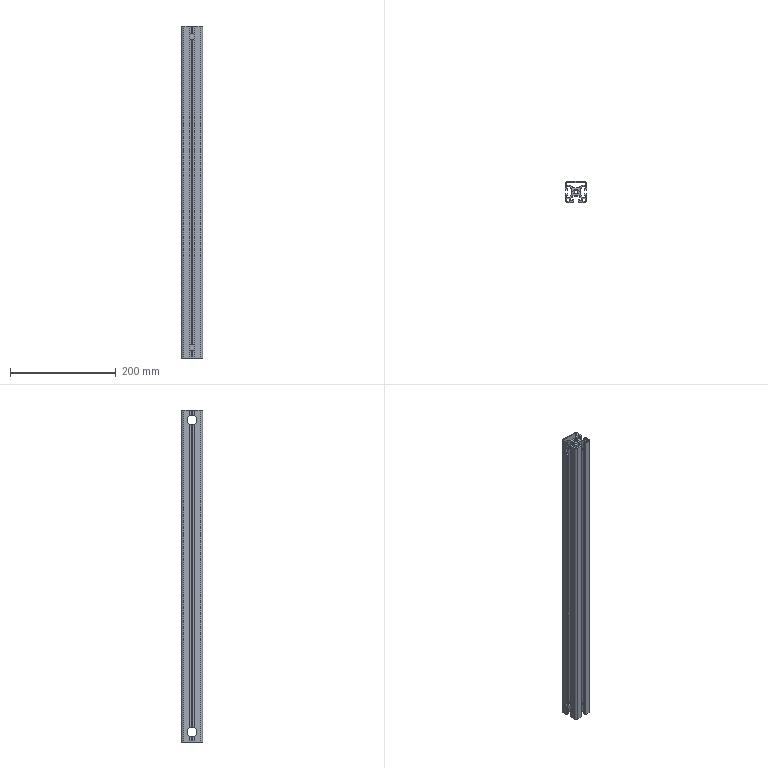Part | SolidWorks | features BaseBody 1, HoleWzd 1, MoveFace 1 | 1 solid | 242 faces | box 40 x 40 x 628 mm | volume 363437 mm3 | plane 187 | cylinder 55 | commonest cylinder face diameters 6.8 x15 2 x14 19 x12 1 x6 5 x4 9 x4